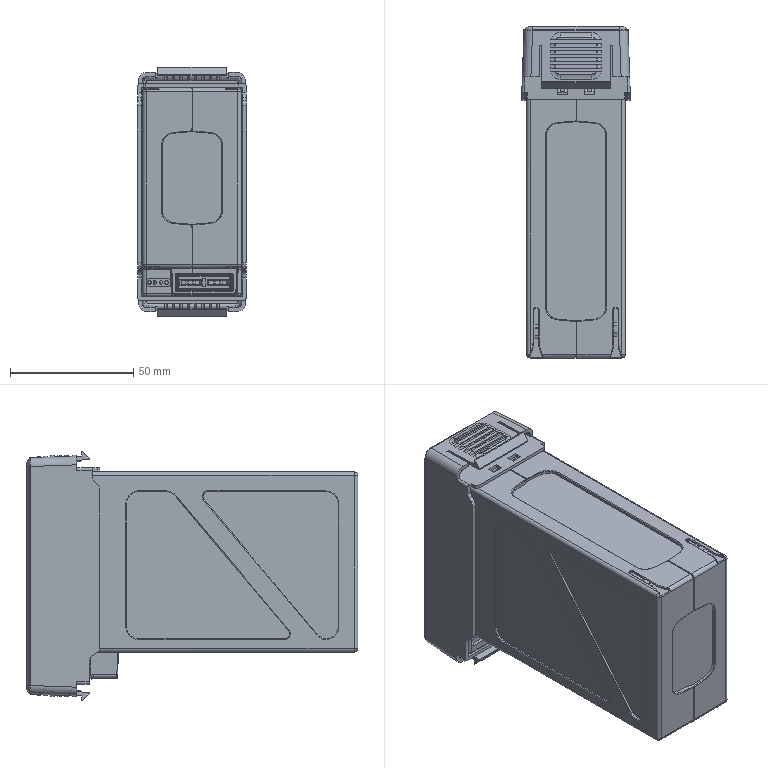Part | SolidWorks | features BaseBody 10 | 11 solids | 2686 faces | box 44.3 x 134.8 x 101.5 mm | volume 316528 mm3 | plane 1716 | cylinder 695 | spline 209 | cone 49 | torus 17 | commonest cylinder face diameters 1 x197 0.6 x84 2 x60 4 x34 0.3 x32 1.3 x32